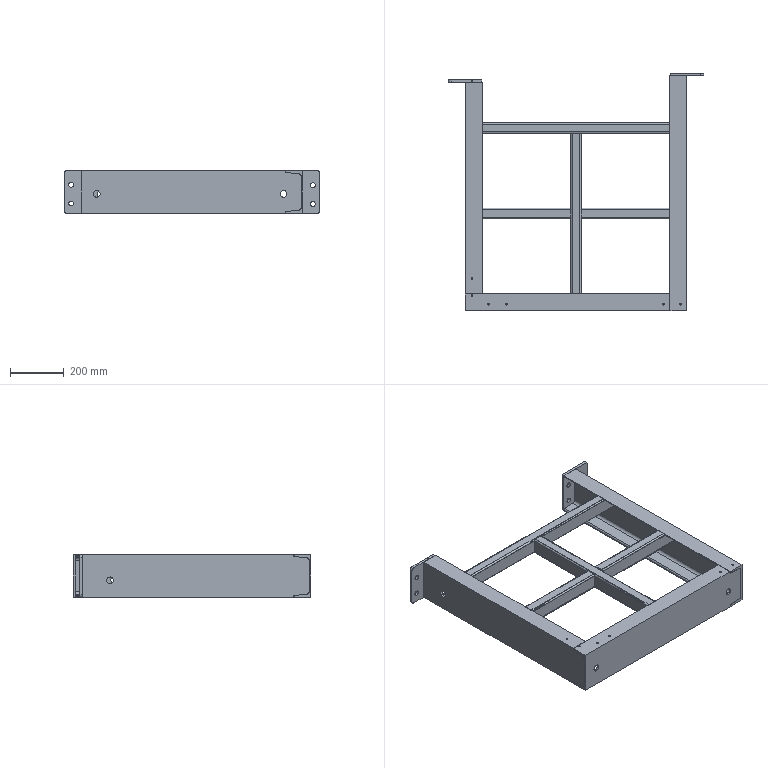Part | STEP file | PN_0044 steel stair platform_Default<As Machined> | 9 solids | 205 faces | box 951 x 886.002 x 160 mm | volume 6916698 mm3 | plane 109 | cylinder 95 | cone 1 | commonest cylinder face diameters 20 x20 6 x16 10 x16 12 x16 18 x14 6.8 x9